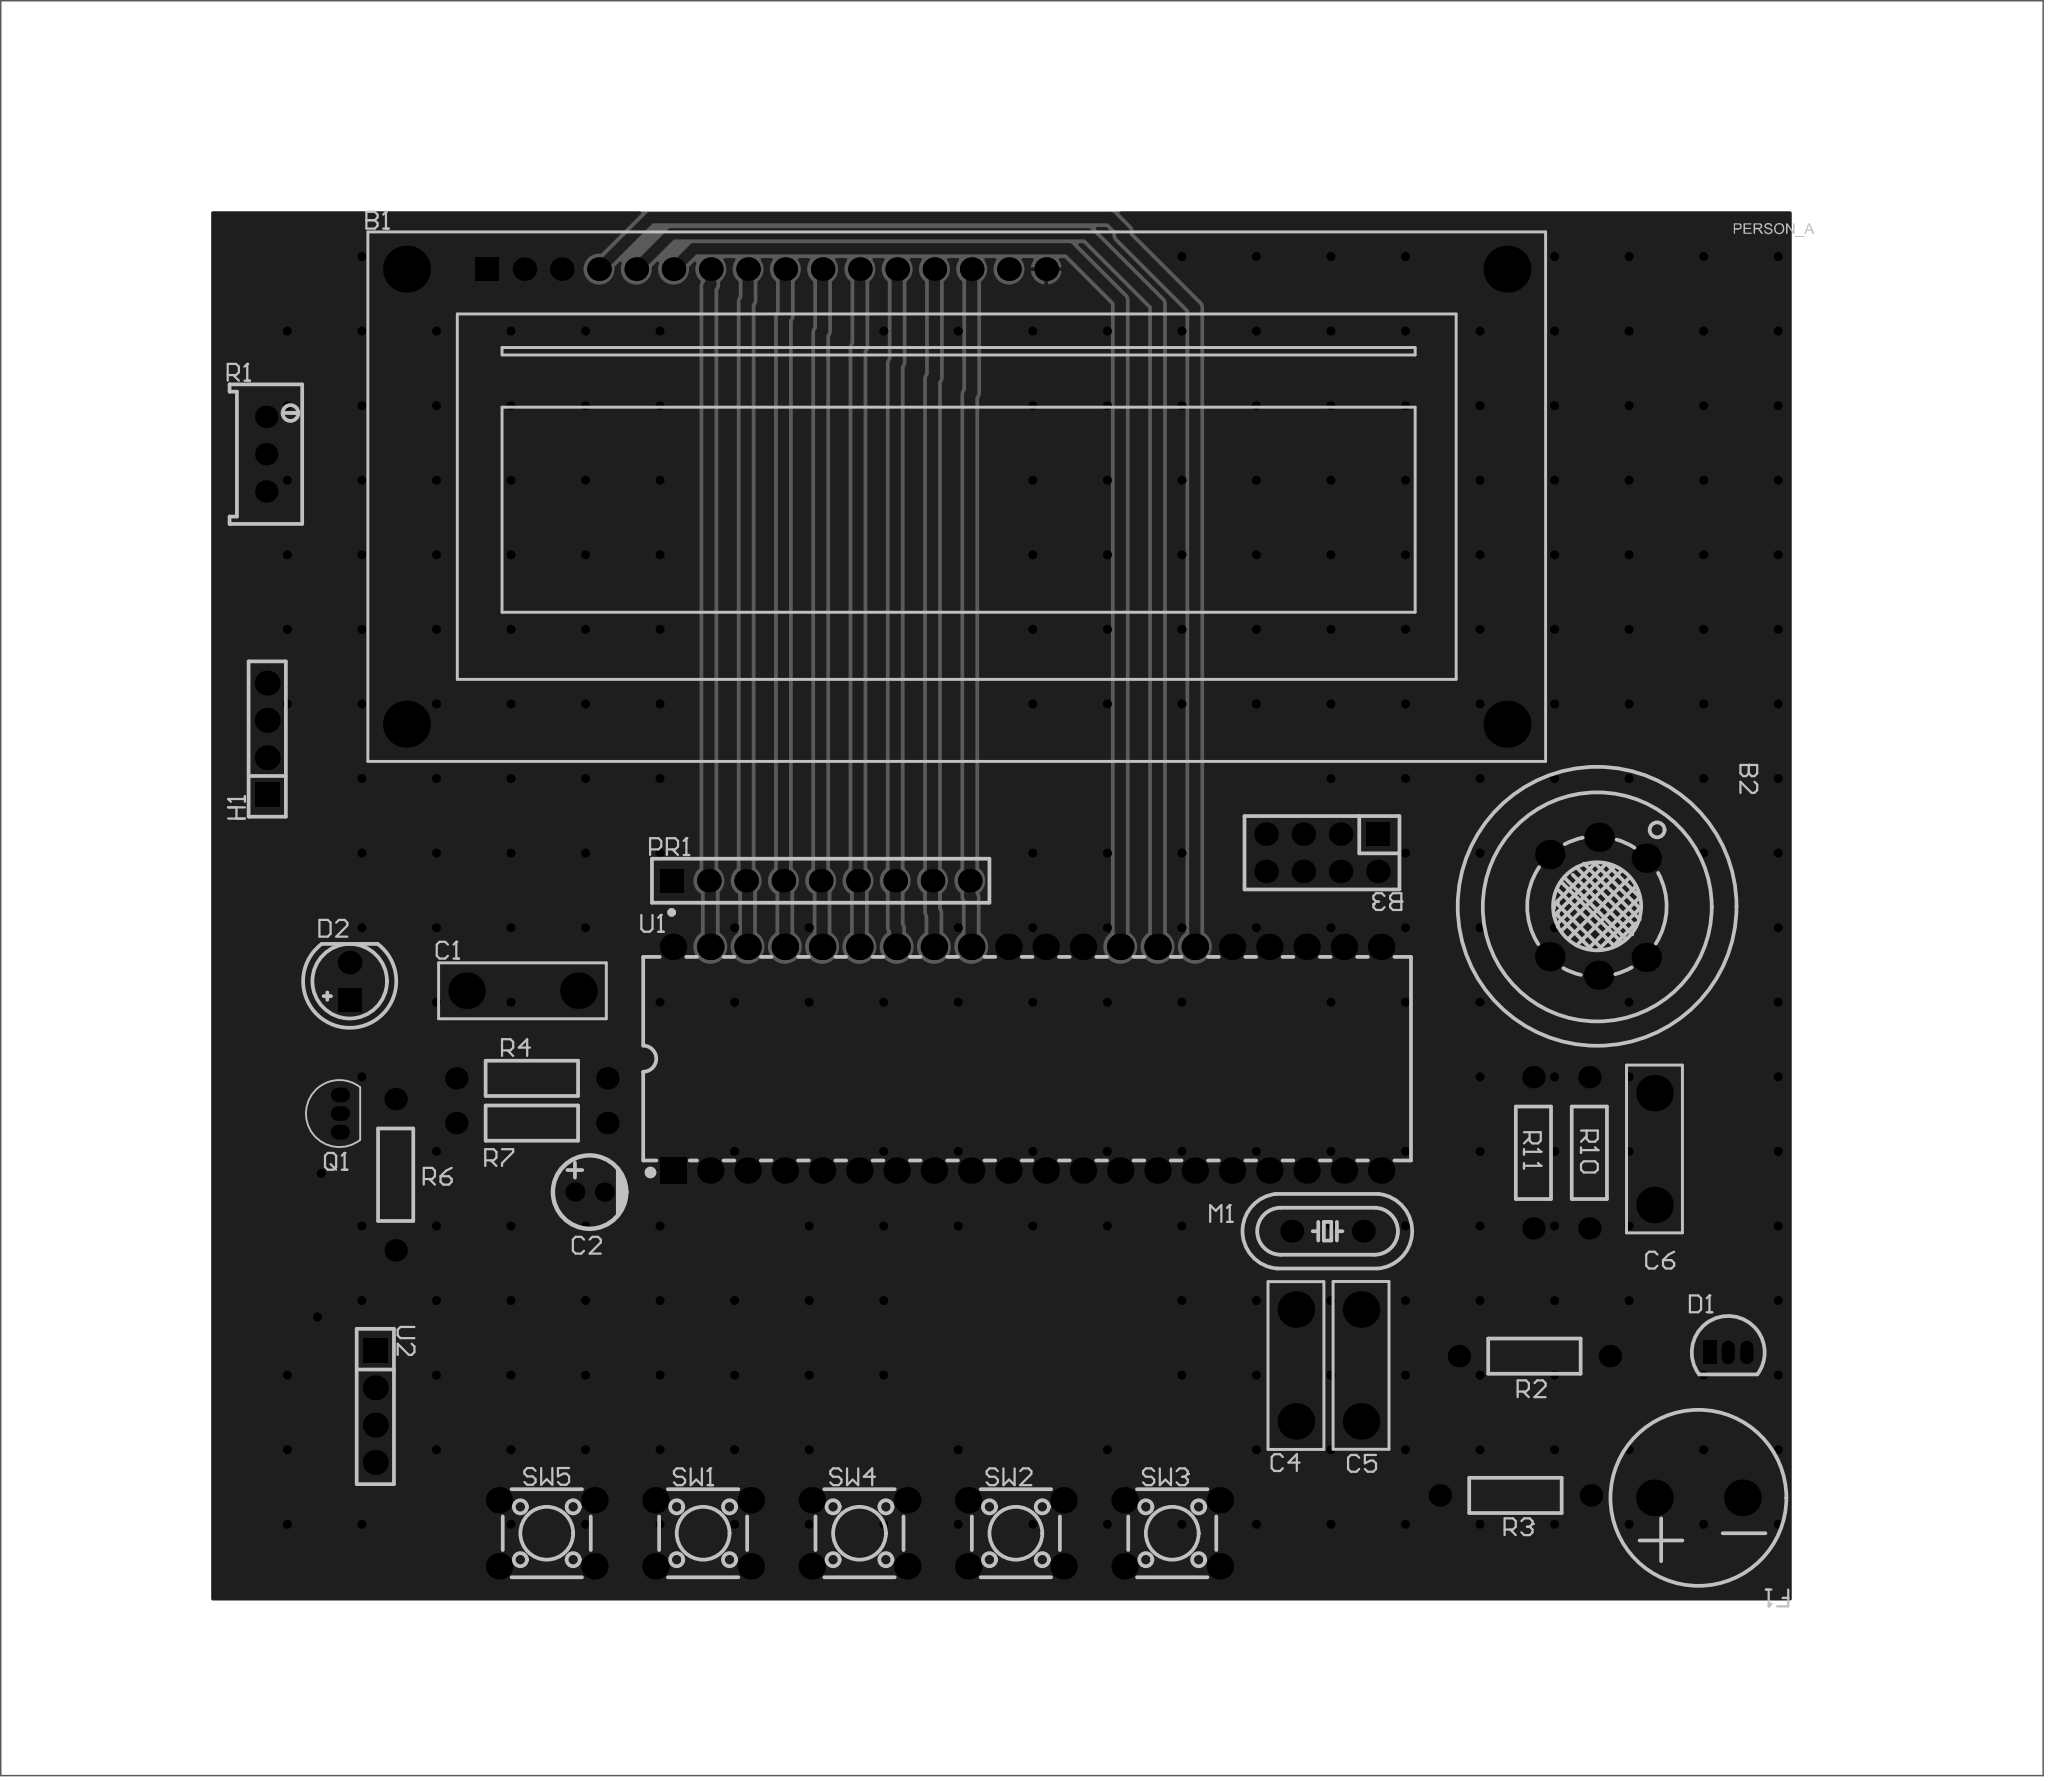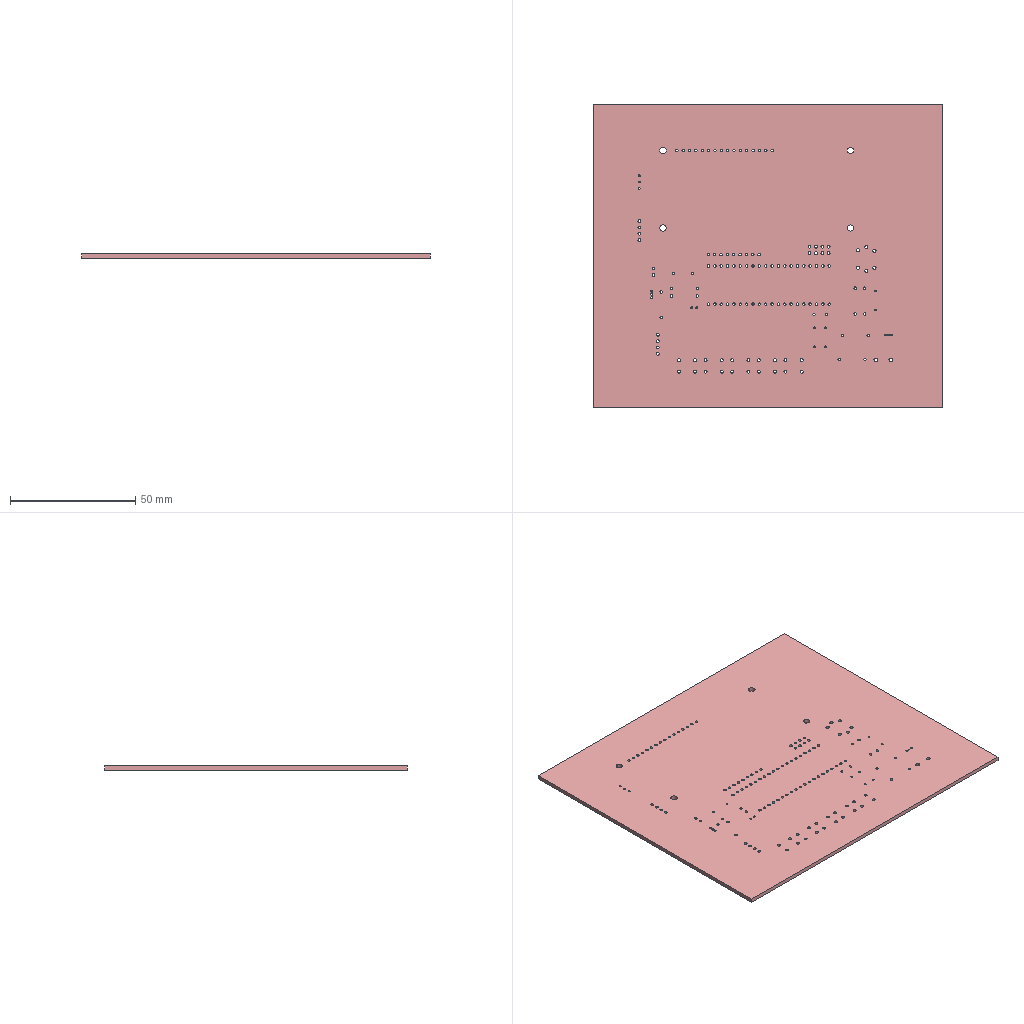Circuit board layout | Altium Designer | box 139.2 x 120.9 x 1.6 mm
Layer stack:
# Altium Designer layer stack of  (unit mm; dielectric type: 0 none, 1 core, 2 prepreg, 3 surface material)
index,name,kind,layer,copper_thickness_mm,dielectric_type,dielectric_thickness_mm,dielectric_material,dielectric_constant
0,Top Paste Mask Layer,other,,,,,,
1,Top Silkscreen Layer,other,,,,,,
2,Top Solder Mask Layer,dielectric,,,3,0.01,,3.3
3,Top Layer,copper,Top Layer,0.035,,,,
4,Dielectric1,dielectric,,,3,1.51,FR4,4.5
5,Bottom Layer,copper,Bottom Layer,0.035,,,,
6,Bottom Solder Mask Layer,dielectric,,,3,0.01,,3.3
7,Bottom Silkscreen Layer,other,,,,,,
8,Bottom Paste Mask Layer,other,,,,,,
# drill layer pairs: low layer,high layer
drill_pair,Top Layer,Bottom Layer
Part placement:
Designator,Comment,Layer,Footprint,Center-X(mm),Center-Y(mm),Rotation
B1,LCD1602,TopLayer,LCD1602,135.001,156.972,0
B2,MQ-2,TopLayer,SENSOR-TH_MQ-2,178.706,129.068,270
B3,DS18B20U+T&R,TopLayer,HDR-TH_8P-P2.54-V-F-R2-C4-S2.54-1,159.893,132.715,180
C1,Cap,TopLayer,RAD-0.3,105.41,123.317,0
C2,Electrolytic capacitor,TopLayer,CAP-TH_BD5.0-P2.00-D0.8-FD-10UF50VC110GL,109.982,109.601,0
C4,Cap,TopLayer,RAD-0.3,158.115,97.79,90
C5,Cap,TopLayer,RAD-0.3,162.56,97.79,270
C6,Cap,TopLayer,RAD-0.3,182.558,112.531,270
D1,PNP transistor,TopLayer,S8550P_TO-92,187.579,98.679,0
D2,LED0,TopLayer,LED-TH_5mm,93.631,123.966,90
F1,Buzzer,TopLayer,BUZ-TH_BD12.0-P6.00-D0.9-RD,185.547,88.773,180
M1,Crystal oscillator,TopLayer,HC-49S_L11.5-W5.0-P4.88,160.274,106.934,0
PR1,8-resistor 9-pin array,TopLayer,RES-ARRAY-TH_9P-P2.54-D1.0,125.73,130.81,0
Q1,PNP,TopLayer,TO-92-3_L4.6-W3.6-P1.27-L_1,92.996,114.949,270
R1,Res Adj2,TopLayer,RES-ADJ-TH_3P-L9.5-W4.85-P2.54_PV36W103C01B00,87.945,159.871,0
R2,?K,TopLayer,Res_1/4W,174.371,98.425,0
R3,?K,TopLayer,Res_1/4W,173.077,88.938,180
R4,?K,TopLayer,Res_1/4W,106.045,117.348,0
R6,?K,TopLayer,Res_1/4W,96.764,110.782,90
R7,?K,TopLayer,Res_1/4W,106.045,114.3,180
R10,?K,TopLayer,Res_1/4W,178.113,112.277,270
R11,?K,TopLayer,Res_1/4W,174.303,112.277,270
SW1,TSW tactile switch,TopLayer,SW-TH_4P-L6.0-W6.0-P4.50-LS6.5,117.718,86.36,0
SW2,TSW tactile switch,TopLayer,SW-TH_4P-L6.0-W6.0-P4.50-LS6.5,139.032,86.36,0
SW3,TSW tactile switch,TopLayer,SW-TH_4P-L6.0-W6.0-P4.50-LS6.5,149.689,86.36,0
SW4,TSW tactile switch,TopLayer,SW-TH_4P-L6.0-W6.0-P4.50-LS6.5,128.375,86.36,0
SW5,TSW tactile switch,TopLayer,SW-TH_4P-L6.0-W6.0-P4.50-LS6.5,107.061,86.36,180
U1,STC12C5A60S2,TopLayer,DIP-40_L52.3-W13.9-P2.54-LS15.2-BL-BASE,139.796,118.687,0
U2,HC05,TopLayer,HDR-TH_4P-P2.54-V-F,95.377,94.996,270
H1,,TopLayer,HDR-TH_4P-P2.54-V-F,88.011,140.462,90
Pad and via stacks:
# Altium Designer via and pad stacks of  (unit mm). Each distinct definition once, with the count of objects using it.
# via: kind,start_layer,end_layer,hole_mm,diameter_mm,mode(0 simple;1 top-mid-bottom;2 full stack),diameter_per_layer,count,example_net
# pad: kind,layer,hole_mm,hole_type(0 round;1 square;2 slot),plating,top_size,top_shape(1 round;2 rect;3 octagon;9 rounded rect),mid_size,bottom_size,mode,footprint,size_per_layer,count,example
pad,Multi-Layer,1,0,plated,1.6x1.6,1,1.6x1.6,1.6x1.6,0,LCD1602,,15,B1.16
pad,Multi-Layer,1,0,plated,1.6x1.6,2,1.6x1.6,1.6x1.6,0,LCD1602,,1,B1.1
pad,Multi-Layer,2.5,2,plated,3.2x3.2,1,3.2x3.2,3.2x3.2,0,LCD1602,,4,B1.0
pad,Multi-Layer,1.3,0,plated,2x2,1,2x2,2x2,0,SENSOR-TH_MQ-2,,6,B2.1
pad,Multi-Layer,1.1,0,plated,1.6x1.6,2,1.6x1.6,1.6x1.6,0,HDR-TH_8P-P2.54-V-F-R2-C4-S2.54-1,,1,B3.1
pad,Multi-Layer,1.1,0,plated,1.6x1.6,1,1.6x1.6,1.6x1.6,0,HDR-TH_8P-P2.54-V-F-R2-C4-S2.54-1,,7,B3.2
pad,Multi-Layer,0.7112,0,plated,2.489x2.489,1,2.489x2.489,2.489x2.489,0,RAD-0.3,,8,C1.2
pad,Multi-Layer,0.8,0,plated,1.3x1.3,1,1.3x1.3,1.3x1.3,0,CAP-TH_BD5.0-P2.00-D0.8-FD-10UF50VC110GL,,2,C2.2
pad,Multi-Layer,0.7,0,plated,0.9x1.6,1,0.9x1.6,0.9x1.6,0,S8550P_TO-92,,2,D1.3
pad,Multi-Layer,0.7,0,plated,0.9x1.6,2,0.9x1.6,0.9x1.6,0,S8550P_TO-92,,1,D1.1
pad,Multi-Layer,1,0,plated,1.6x1.6,2,1.6x1.6,1.6x1.6,0,LED-TH_5mm,,1,D2.1
pad,Multi-Layer,1,0,plated,1.6x1.6,1,1.6x1.6,1.6x1.6,0,LED-TH_5mm,,1,D2.2
pad,Multi-Layer,1.5,0,plated,2.5x2.5,1,2.5x2.5,2.5x2.5,0,BUZ-TH_BD12.0-P6.00-D0.9-RD,,2,F1.1
pad,Multi-Layer,0.9,0,plated,1.56x1.56,1,1.56x1.56,1.56x1.56,0,HC-49S_L11.5-W5.0-P4.88,,2,M1.1
pad,Multi-Layer,1,0,plated,1.6x1.6,2,1.6x1.6,1.6x1.6,0,RES-ARRAY-TH_9P-P2.54-D1.0,,1,PR1.1
pad,Multi-Layer,1,0,plated,1.6x1.6,1,1.6x1.6,1.6x1.6,0,RES-ARRAY-TH_9P-P2.54-D1.0,,8,PR1.2
pad,Multi-Layer,0.8,2,plated,1x1.3,1,1x1.3,1x1.3,0,TO-92-3_L4.6-W3.6-P1.27-L_1,,3,Q1.1
pad,Multi-Layer,0.762,0,plated,1.524x1.524,1,1.524x1.524,1.524x1.524,0,RES-ADJ-TH_3P-L9.5-W4.85-P2.54_PV36W103C01B00,,3,R1.3
pad,Multi-Layer,1,0,plated,1.524x1.524,1,1.524x1.524,1.524x1.524,0,Res_1/4W,,14,R2.1
pad,Multi-Layer,1.2,0,plated,1.8x1.8,1,1.8x1.8,1.8x1.8,0,SW-TH_4P-L6.0-W6.0-P4.50-LS6.5,,20,SW1.1
pad,Multi-Layer,1,0,plated,1.8x1.8,1,1.8x1.8,1.8x1.8,0,DIP-40_L52.3-W13.9-P2.54-LS15.2-BL-BASE,,39,U1.36
pad,Multi-Layer,1,0,plated,1.8x1.8,2,1.8x1.8,1.8x1.8,0,DIP-40_L52.3-W13.9-P2.54-LS15.2-BL-BASE,,1,U1.1
pad,Multi-Layer,1.1,0,plated,1.7x1.7,2,1.7x1.7,1.7x1.7,0,HDR-TH_4P-P2.54-V-F,,2,U2.1
pad,Multi-Layer,1.1,0,plated,1.7x1.7,1,1.7x1.7,1.7x1.7,0,HDR-TH_4P-P2.54-V-F,,6,U2.2
via,Top Layer,Bottom Layer,0.3048,0.61,0,,275,P12
Copper pours:
name,layer,net,type(0 solid;1 hatched;2 none)
Bottom Layer-GND,Bottom Layer,GND,0
Top Layer-GND,Top Layer,GND,0